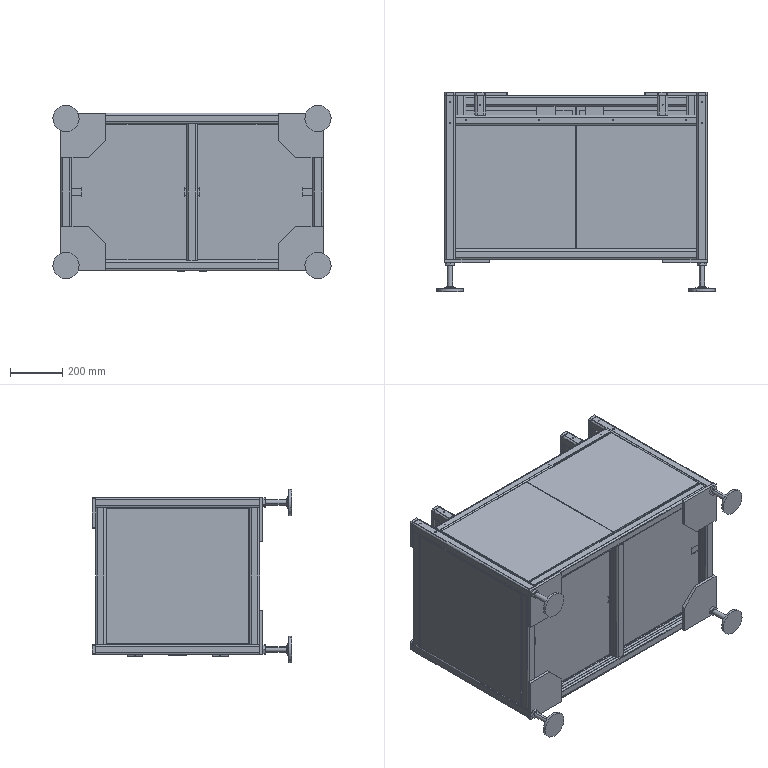Part | SolidWorks | features Cut 1 | 49 solids | 1082 faces | box 1060 x 759 x 660 mm | volume 11116093 mm3 | plane 638 | cylinder 420 | sphere 16 | cone 8 | commonest cylinder face diameters 8 x120 16 x100 5 x60 15 x28 10 x20 1 x16